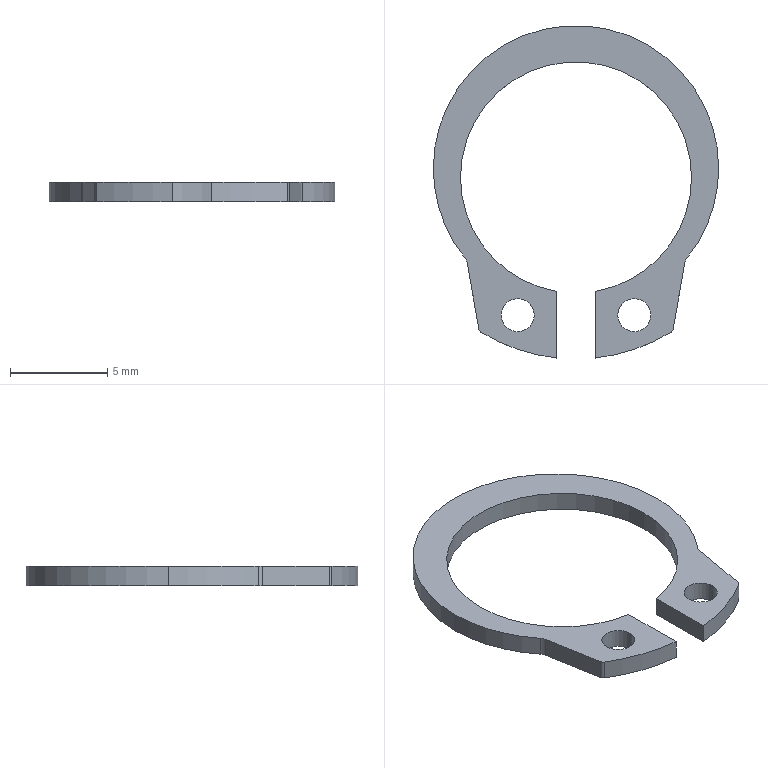Part | SolidWorks | features Extrusion 1 | 1 solid | 22 faces | box 14.7 x 17.116 x 1 mm | volume 75.123 mm3 | cylinder 16 | plane 6 | commonest cylinder face diameters 1.7 x4 11.9 x3 14.7 x3 0.4 x2 1 x2 18.7 x2
STEP:
#1=CARTESIAN_POINT('',(2.15,-7.562,0.5));
#2=VERTEX_POINT('',#1);
#3=CARTESIAN_POINT('',(3.85,-7.562,0.5));
#4=VERTEX_POINT('',#3);
#5=CARTESIAN_POINT('',(3.,-7.562,0.5));
#6=DIRECTION('',(0.,0.,1.));
#7=DIRECTION('',(-1.,0.,0.));
#8=AXIS2_PLACEMENT_3D('',#5,#6,#7);
#9=CIRCLE('',#8,0.85);
#10=EDGE_CURVE('',#2,#4,#9,.T.);
#11=ORIENTED_EDGE('',*,*,#10,.T.);
#12=CARTESIAN_POINT('',(3.85,-7.562,-0.5));
#13=VERTEX_POINT('',#12);
#14=CARTESIAN_POINT('',(3.85,-7.562,0.5));
#15=DIRECTION('',(0.,0.,-1.));
#16=VECTOR('',#15,1000.);
#17=LINE('',#14,#16);
#18=EDGE_CURVE('',#4,#13,#17,.T.);
#19=ORIENTED_EDGE('',*,*,#18,.T.);
#20=CARTESIAN_POINT('',(2.15,-7.562,-0.5));
#21=VERTEX_POINT('',#20);
#22=CARTESIAN_POINT('',(3.,-7.562,-0.5));
#23=DIRECTION('',(0.,0.,1.));
#24=DIRECTION('',(-1.,0.,0.));
#25=AXIS2_PLACEMENT_3D('',#22,#23,#24);
#26=CIRCLE('',#25,0.85);
#27=EDGE_CURVE('',#21,#13,#26,.T.);
#28=ORIENTED_EDGE('',*,*,#27,.F.);
#29=CARTESIAN_POINT('',(2.15,-7.562,0.5));
#30=DIRECTION('',(0.,0.,-1.));
#31=VECTOR('',#30,1000.);
#32=LINE('',#29,#31);
#33=EDGE_CURVE('',#2,#21,#32,.T.);
#34=ORIENTED_EDGE('',*,*,#33,.F.);
#35=EDGE_LOOP('',(#11,#19,#28,#34));
#36=FACE_OUTER_BOUND('',#35,.T.);
#37=CARTESIAN_POINT('',(3.,-7.562,0.5));
#38=DIRECTION('',(0.,0.,-1.));
#39=DIRECTION('',(-1.,0.,0.));
#40=AXIS2_PLACEMENT_3D('',#37,#38,#39);
#41=CYLINDRICAL_SURFACE('',#40,0.85);
#42=ADVANCED_FACE('',(#36),#41,.F.);
#43=CARTESIAN_POINT('',(-3.85,-7.562,0.5));
#44=VERTEX_POINT('',#43);
#45=CARTESIAN_POINT('',(-2.15,-7.562,0.5));
#46=VERTEX_POINT('',#45);
#47=CARTESIAN_POINT('',(-3.,-7.562,0.5));
#48=DIRECTION('',(0.,0.,1.));
#49=DIRECTION('',(1.,0.,0.));
#50=AXIS2_PLACEMENT_3D('',#47,#48,#49);
#51=CIRCLE('',#50,0.85);
#52=EDGE_CURVE('',#44,#46,#51,.T.);
#53=ORIENTED_EDGE('',*,*,#52,.T.);
#54=CARTESIAN_POINT('',(-2.15,-7.562,-0.5));
#55=VERTEX_POINT('',#54);
#56=CARTESIAN_POINT('',(-2.15,-7.562,0.5));
#57=DIRECTION('',(0.,0.,-1.));
#58=VECTOR('',#57,1000.);
#59=LINE('',#56,#58);
#60=EDGE_CURVE('',#46,#55,#59,.T.);
#61=ORIENTED_EDGE('',*,*,#60,.T.);
#62=CARTESIAN_POINT('',(-3.85,-7.562,-0.5));
#63=VERTEX_POINT('',#62);
#64=CARTESIAN_POINT('',(-3.,-7.562,-0.5));
#65=DIRECTION('',(0.,0.,1.));
#66=DIRECTION('',(1.,0.,0.));
#67=AXIS2_PLACEMENT_3D('',#64,#65,#66);
#68=CIRCLE('',#67,0.85);
#69=EDGE_CURVE('',#63,#55,#68,.T.);
#70=ORIENTED_EDGE('',*,*,#69,.F.);
#71=CARTESIAN_POINT('',(-3.85,-7.562,0.5));
#72=DIRECTION('',(0.,0.,-1.));
#73=VECTOR('',#72,1000.);
#74=LINE('',#71,#73);
#75=EDGE_CURVE('',#44,#63,#74,.T.);
#76=ORIENTED_EDGE('',*,*,#75,.F.);
#77=EDGE_LOOP('',(#53,#61,#70,#76));
#78=FACE_OUTER_BOUND('',#77,.T.);
#79=CARTESIAN_POINT('',(-3.,-7.562,0.5));
#80=DIRECTION('',(0.,0.,-1.));
#81=DIRECTION('',(-1.,0.,0.));
#82=AXIS2_PLACEMENT_3D('',#79,#80,#81);
#83=CYLINDRICAL_SURFACE('',#82,0.85);
#84=ADVANCED_FACE('',(#78),#83,.F.);
#85=CARTESIAN_POINT('',(7.35,0.,0.5));
#86=VERTEX_POINT('',#85);
#87=CARTESIAN_POINT('',(-7.35,0.,0.5));
#88=VERTEX_POINT('',#87);
#89=CARTESIAN_POINT('',(0.,0.,0.5));
#90=DIRECTION('',(0.,0.,1.));
#91=DIRECTION('',(1.,0.,0.));
#92=AXIS2_PLACEMENT_3D('',#89,#90,#91);
#93=CIRCLE('',#92,7.35);
#94=EDGE_CURVE('',#86,#88,#93,.T.);
#95=ORIENTED_EDGE('',*,*,#94,.F.);
#96=CARTESIAN_POINT('',(7.35,0.,-0.5));
#97=VERTEX_POINT('',#96);
#98=CARTESIAN_POINT('',(7.35,0.,0.5));
#99=DIRECTION('',(0.,0.,-1.));
#100=VECTOR('',#99,1000.);
#101=LINE('',#98,#100);
#102=EDGE_CURVE('',#86,#97,#101,.T.);
#103=ORIENTED_EDGE('',*,*,#102,.T.);
#104=CARTESIAN_POINT('',(-7.35,0.,-0.5));
#105=VERTEX_POINT('',#104);
#106=CARTESIAN_POINT('',(0.,0.,-0.5));
#107=DIRECTION('',(0.,0.,1.));
#108=DIRECTION('',(1.,0.,0.));
#109=AXIS2_PLACEMENT_3D('',#106,#107,#108);
#110=CIRCLE('',#109,7.35);
#111=EDGE_CURVE('',#97,#105,#110,.T.);
#112=ORIENTED_EDGE('',*,*,#111,.T.);
#113=CARTESIAN_POINT('',(-7.35,0.,0.5));
#114=DIRECTION('',(0.,0.,-1.));
#115=VECTOR('',#114,1000.);
#116=LINE('',#113,#115);
#117=EDGE_CURVE('',#88,#105,#116,.T.);
#118=ORIENTED_EDGE('',*,*,#117,.F.);
#119=EDGE_LOOP('',(#95,#103,#112,#118));
#120=FACE_OUTER_BOUND('',#119,.T.);
#121=CARTESIAN_POINT('',(0.,0.,0.5));
#122=DIRECTION('',(0.,0.,-1.));
#123=DIRECTION('',(-1.,0.,0.));
#124=AXIS2_PLACEMENT_3D('',#121,#122,#123);
#125=CYLINDRICAL_SURFACE('',#124,7.35);
#126=ADVANCED_FACE('',(#120),#125,.T.);
#127=CARTESIAN_POINT('',(-5.71,-4.628,0.5));
#128=VERTEX_POINT('',#127);
#129=CARTESIAN_POINT('',(0.,0.,0.5));
#130=DIRECTION('',(0.,0.,1.));
#131=DIRECTION('',(1.,0.,0.));
#132=AXIS2_PLACEMENT_3D('',#129,#130,#131);
#133=CIRCLE('',#132,7.35);
#134=EDGE_CURVE('',#88,#128,#133,.T.);
#135=ORIENTED_EDGE('',*,*,#134,.F.);
#136=ORIENTED_EDGE('',*,*,#117,.T.);
#137=CARTESIAN_POINT('',(-5.71,-4.628,-0.5));
#138=VERTEX_POINT('',#137);
#139=CARTESIAN_POINT('',(0.,0.,-0.5));
#140=DIRECTION('',(0.,0.,1.));
#141=DIRECTION('',(1.,0.,0.));
#142=AXIS2_PLACEMENT_3D('',#139,#140,#141);
#143=CIRCLE('',#142,7.35);
#144=EDGE_CURVE('',#105,#138,#143,.T.);
#145=ORIENTED_EDGE('',*,*,#144,.T.);
#146=CARTESIAN_POINT('',(-5.71,-4.628,0.5));
#147=DIRECTION('',(0.,0.,-1.));
#148=VECTOR('',#147,1000.);
#149=LINE('',#146,#148);
#150=EDGE_CURVE('',#128,#138,#149,.T.);
#151=ORIENTED_EDGE('',*,*,#150,.F.);
#152=EDGE_LOOP('',(#135,#136,#145,#151));
#153=FACE_OUTER_BOUND('',#152,.T.);
#154=CARTESIAN_POINT('',(0.,0.,0.5));
#155=DIRECTION('',(0.,0.,-1.));
#156=DIRECTION('',(-1.,0.,0.));
#157=AXIS2_PLACEMENT_3D('',#154,#155,#156);
#158=CYLINDRICAL_SURFACE('',#157,7.35);
#159=ADVANCED_FACE('',(#153),#158,.T.);
#160=CARTESIAN_POINT('',(5.95,-0.47,0.5));
#161=VERTEX_POINT('',#160);
#162=CARTESIAN_POINT('',(1.,-6.335,0.5));
#163=VERTEX_POINT('',#162);
#164=CARTESIAN_POINT('',(0.,-0.47,0.5));
#165=DIRECTION('',(0.,0.,-1.));
#166=DIRECTION('',(1.,0.,0.));
#167=AXIS2_PLACEMENT_3D('',#164,#165,#166);
#168=CIRCLE('',#167,5.95);
#169=EDGE_CURVE('',#161,#163,#168,.T.);
#170=ORIENTED_EDGE('',*,*,#169,.F.);
#171=CARTESIAN_POINT('',(5.95,-0.47,-0.5));
#172=VERTEX_POINT('',#171);
#173=CARTESIAN_POINT('',(5.95,-0.47,0.5));
#174=DIRECTION('',(0.,0.,-1.));
#175=VECTOR('',#174,1000.);
#176=LINE('',#173,#175);
#177=EDGE_CURVE('',#161,#172,#176,.T.);
#178=ORIENTED_EDGE('',*,*,#177,.T.);
#179=CARTESIAN_POINT('',(1.,-6.335,-0.5));
#180=VERTEX_POINT('',#179);
#181=CARTESIAN_POINT('',(0.,-0.47,-0.5));
#182=DIRECTION('',(0.,0.,-1.));
#183=DIRECTION('',(1.,0.,0.));
#184=AXIS2_PLACEMENT_3D('',#181,#182,#183);
#185=CIRCLE('',#184,5.95);
#186=EDGE_CURVE('',#172,#180,#185,.T.);
#187=ORIENTED_EDGE('',*,*,#186,.T.);
#188=CARTESIAN_POINT('',(1.,-6.335,0.5));
#189=DIRECTION('',(0.,0.,-1.));
#190=VECTOR('',#189,1000.);
#191=LINE('',#188,#190);
#192=EDGE_CURVE('',#163,#180,#191,.T.);
#193=ORIENTED_EDGE('',*,*,#192,.F.);
#194=EDGE_LOOP('',(#170,#178,#187,#193));
#195=FACE_OUTER_BOUND('',#194,.T.);
#196=CARTESIAN_POINT('',(0.,-0.47,0.5));
#197=DIRECTION('',(0.,0.,-1.));
#198=DIRECTION('',(-1.,0.,0.));
#199=AXIS2_PLACEMENT_3D('',#196,#197,#198);
#200=CYLINDRICAL_SURFACE('',#199,5.95);
#201=ADVANCED_FACE('',(#195),#200,.F.);
#202=ORIENTED_EDGE('',*,*,#177,.F.);
#203=CARTESIAN_POINT('',(-5.95,-0.47,0.5));
#204=VERTEX_POINT('',#203);
#205=CARTESIAN_POINT('',(0.,-0.47,0.5));
#206=DIRECTION('',(0.,0.,-1.));
#207=DIRECTION('',(1.,0.,0.));
#208=AXIS2_PLACEMENT_3D('',#205,#206,#207);
#209=CIRCLE('',#208,5.95);
#210=EDGE_CURVE('',#204,#161,#209,.T.);
#211=ORIENTED_EDGE('',*,*,#210,.F.);
#212=CARTESIAN_POINT('',(-5.95,-0.47,-0.5));
#213=VERTEX_POINT('',#212);
#214=CARTESIAN_POINT('',(-5.95,-0.47,0.5));
#215=DIRECTION('',(0.,0.,-1.));
#216=VECTOR('',#215,1000.);
#217=LINE('',#214,#216);
#218=EDGE_CURVE('',#204,#213,#217,.T.);
#219=ORIENTED_EDGE('',*,*,#218,.T.);
#220=CARTESIAN_POINT('',(0.,-0.47,-0.5));
#221=DIRECTION('',(0.,0.,-1.));
#222=DIRECTION('',(1.,0.,0.));
#223=AXIS2_PLACEMENT_3D('',#220,#221,#222);
#224=CIRCLE('',#223,5.95);
#225=EDGE_CURVE('',#213,#172,#224,.T.);
#226=ORIENTED_EDGE('',*,*,#225,.T.);
#227=EDGE_LOOP('',(#202,#211,#219,#226));
#228=FACE_OUTER_BOUND('',#227,.T.);
#229=CARTESIAN_POINT('',(0.,-0.47,0.5));
#230=DIRECTION('',(0.,0.,-1.));
#231=DIRECTION('',(-1.,0.,0.));
#232=AXIS2_PLACEMENT_3D('',#229,#230,#231);
#233=CYLINDRICAL_SURFACE('',#232,5.95);
#234=ADVANCED_FACE('',(#228),#233,.F.);
#235=ORIENTED_EDGE('',*,*,#52,.F.);
#236=CARTESIAN_POINT('',(-3.,-7.562,0.5));
#237=DIRECTION('',(0.,0.,1.));
#238=DIRECTION('',(1.,0.,0.));
#239=AXIS2_PLACEMENT_3D('',#236,#237,#238);
#240=CIRCLE('',#239,0.85);
#241=EDGE_CURVE('',#46,#44,#240,.T.);
#242=ORIENTED_EDGE('',*,*,#241,.F.);
#243=EDGE_LOOP('',(#235,#242));
#244=FACE_BOUND('',#243,.T.);
#245=CARTESIAN_POINT('',(-5.606,-4.856,0.5));
#246=VERTEX_POINT('',#245);
#247=CARTESIAN_POINT('',(-6.098,-4.943,0.5));
#248=DIRECTION('',(0.,0.,-1.));
#249=DIRECTION('',(1.,0.,0.));
#250=AXIS2_PLACEMENT_3D('',#247,#248,#249);
#251=CIRCLE('',#250,0.5);
#252=EDGE_CURVE('',#128,#246,#251,.T.);
#253=ORIENTED_EDGE('',*,*,#252,.T.);
#254=CARTESIAN_POINT('',(-5.,-8.293,0.5));
#255=VERTEX_POINT('',#254);
#256=CARTESIAN_POINT('',(-5.606,-4.856,0.5));
#257=DIRECTION('',(0.1736,-0.9848,0.));
#258=VECTOR('',#257,1000.);
#259=LINE('',#256,#258);
#260=EDGE_CURVE('',#246,#255,#259,.T.);
#261=ORIENTED_EDGE('',*,*,#260,.T.);
#262=CARTESIAN_POINT('',(-4.908,-8.428,0.5));
#263=VERTEX_POINT('',#262);
#264=CARTESIAN_POINT('',(-4.803,-8.258,0.5));
#265=DIRECTION('',(0.,0.,1.));
#266=DIRECTION('',(-1.,0.,0.));
#267=AXIS2_PLACEMENT_3D('',#264,#265,#266);
#268=CIRCLE('',#267,0.2);
#269=EDGE_CURVE('',#255,#263,#268,.T.);
#270=ORIENTED_EDGE('',*,*,#269,.T.);
#271=CARTESIAN_POINT('',(-1.,-9.766,0.5));
#272=VERTEX_POINT('',#271);
#273=CARTESIAN_POINT('',(0.,-0.47,0.5));
#274=DIRECTION('',(0.,0.,1.));
#275=DIRECTION('',(-1.,0.,0.));
#276=AXIS2_PLACEMENT_3D('',#273,#274,#275);
#277=CIRCLE('',#276,9.35);
#278=EDGE_CURVE('',#263,#272,#277,.T.);
#279=ORIENTED_EDGE('',*,*,#278,.T.);
#280=CARTESIAN_POINT('',(-1.,-6.335,0.5));
#281=VERTEX_POINT('',#280);
#282=CARTESIAN_POINT('',(-1.,-6.335,0.5));
#283=DIRECTION('',(0.,1.,0.));
#284=VECTOR('',#283,1000.);
#285=LINE('',#282,#284);
#286=EDGE_CURVE('',#272,#281,#285,.T.);
#287=ORIENTED_EDGE('',*,*,#286,.T.);
#288=CARTESIAN_POINT('',(0.,-0.47,0.5));
#289=DIRECTION('',(0.,0.,-1.));
#290=DIRECTION('',(1.,0.,0.));
#291=AXIS2_PLACEMENT_3D('',#288,#289,#290);
#292=CIRCLE('',#291,5.95);
#293=EDGE_CURVE('',#281,#204,#292,.T.);
#294=ORIENTED_EDGE('',*,*,#293,.T.);
#295=ORIENTED_EDGE('',*,*,#210,.T.);
#296=ORIENTED_EDGE('',*,*,#169,.T.);
#297=CARTESIAN_POINT('',(1.,-9.766,0.5));
#298=VERTEX_POINT('',#297);
#299=CARTESIAN_POINT('',(1.,-6.335,0.5));
#300=DIRECTION('',(0.,-1.,0.));
#301=VECTOR('',#300,1000.);
#302=LINE('',#299,#301);
#303=EDGE_CURVE('',#163,#298,#302,.T.);
#304=ORIENTED_EDGE('',*,*,#303,.T.);
#305=CARTESIAN_POINT('',(4.908,-8.428,0.5));
#306=VERTEX_POINT('',#305);
#307=CARTESIAN_POINT('',(0.,-0.47,0.5));
#308=DIRECTION('',(0.,0.,1.));
#309=DIRECTION('',(1.,0.,0.));
#310=AXIS2_PLACEMENT_3D('',#307,#308,#309);
#311=CIRCLE('',#310,9.35);
#312=EDGE_CURVE('',#298,#306,#311,.T.);
#313=ORIENTED_EDGE('',*,*,#312,.T.);
#314=CARTESIAN_POINT('',(5.,-8.293,0.5));
#315=VERTEX_POINT('',#314);
#316=CARTESIAN_POINT('',(4.803,-8.258,0.5));
#317=DIRECTION('',(0.,0.,1.));
#318=DIRECTION('',(1.,0.,0.));
#319=AXIS2_PLACEMENT_3D('',#316,#317,#318);
#320=CIRCLE('',#319,0.2);
#321=EDGE_CURVE('',#306,#315,#320,.T.);
#322=ORIENTED_EDGE('',*,*,#321,.T.);
#323=CARTESIAN_POINT('',(5.606,-4.856,0.5));
#324=VERTEX_POINT('',#323);
#325=CARTESIAN_POINT('',(5.606,-4.856,0.5));
#326=DIRECTION('',(0.1736,0.9848,0.));
#327=VECTOR('',#326,1000.);
#328=LINE('',#325,#327);
#329=EDGE_CURVE('',#315,#324,#328,.T.);
#330=ORIENTED_EDGE('',*,*,#329,.T.);
#331=CARTESIAN_POINT('',(5.71,-4.628,0.5));
#332=VERTEX_POINT('',#331);
#333=CARTESIAN_POINT('',(6.098,-4.943,0.5));
#334=DIRECTION('',(0.,0.,-1.));
#335=DIRECTION('',(-1.,0.,0.));
#336=AXIS2_PLACEMENT_3D('',#333,#334,#335);
#337=CIRCLE('',#336,0.5);
#338=EDGE_CURVE('',#324,#332,#337,.T.);
#339=ORIENTED_EDGE('',*,*,#338,.T.);
#340=CARTESIAN_POINT('',(0.,0.,0.5));
#341=DIRECTION('',(0.,0.,1.));
#342=DIRECTION('',(1.,0.,0.));
#343=AXIS2_PLACEMENT_3D('',#340,#341,#342);
#344=CIRCLE('',#343,7.35);
#345=EDGE_CURVE('',#332,#86,#344,.T.);
#346=ORIENTED_EDGE('',*,*,#345,.T.);
#347=ORIENTED_EDGE('',*,*,#94,.T.);
#348=ORIENTED_EDGE('',*,*,#134,.T.);
#349=EDGE_LOOP('',(#253,#261,#270,#279,#287,#294,#295,#296,#304,#313,#322,#330,#339,#346,#347,#348));
#350=FACE_OUTER_BOUND('',#349,.T.);
#351=ORIENTED_EDGE('',*,*,#10,.F.);
#352=CARTESIAN_POINT('',(3.,-7.562,0.5));
#353=DIRECTION('',(0.,0.,1.));
#354=DIRECTION('',(-1.,0.,0.));
#355=AXIS2_PLACEMENT_3D('',#352,#353,#354);
#356=CIRCLE('',#355,0.85);
#357=EDGE_CURVE('',#4,#2,#356,.T.);
#358=ORIENTED_EDGE('',*,*,#357,.F.);
#359=EDGE_LOOP('',(#351,#358));
#360=FACE_BOUND('',#359,.T.);
#361=CARTESIAN_POINT('',(-6.098,-4.943,0.5));
#362=DIRECTION('',(0.,0.,1.));
#363=DIRECTION('',(1.,0.,0.));
#364=AXIS2_PLACEMENT_3D('',#361,#362,#363);
#365=PLANE('',#364);
#366=ADVANCED_FACE('',(#244,#350,#360),#365,.T.);
#367=ORIENTED_EDGE('',*,*,#150,.T.);
#368=CARTESIAN_POINT('',(-5.606,-4.856,-0.5));
#369=VERTEX_POINT('',#368);
#370=CARTESIAN_POINT('',(-6.098,-4.943,-0.5));
#371=DIRECTION('',(0.,0.,-1.));
#372=DIRECTION('',(1.,0.,0.));
#373=AXIS2_PLACEMENT_3D('',#370,#371,#372);
#374=CIRCLE('',#373,0.5);
#375=EDGE_CURVE('',#138,#369,#374,.T.);
#376=ORIENTED_EDGE('',*,*,#375,.T.);
#377=CARTESIAN_POINT('',(-5.606,-4.856,0.5));
#378=DIRECTION('',(0.,0.,-1.));
#379=VECTOR('',#378,1000.);
#380=LINE('',#377,#379);
#381=EDGE_CURVE('',#246,#369,#380,.T.);
#382=ORIENTED_EDGE('',*,*,#381,.F.);
#383=ORIENTED_EDGE('',*,*,#252,.F.);
#384=EDGE_LOOP('',(#367,#376,#382,#383));
#385=FACE_OUTER_BOUND('',#384,.T.);
#386=CARTESIAN_POINT('',(-6.098,-4.943,0.5));
#387=DIRECTION('',(0.,0.,-1.));
#388=DIRECTION('',(-1.,0.,0.));
#389=AXIS2_PLACEMENT_3D('',#386,#387,#388);
#390=CYLINDRICAL_SURFACE('',#389,0.5);
#391=ADVANCED_FACE('',(#385),#390,.F.);
#392=ORIENTED_EDGE('',*,*,#381,.T.);
#393=CARTESIAN_POINT('',(-5.,-8.293,-0.5));
#394=VERTEX_POINT('',#393);
#395=CARTESIAN_POINT('',(-5.606,-4.856,-0.5));
#396=DIRECTION('',(0.1736,-0.9848,0.));
#397=VECTOR('',#396,1000.);
#398=LINE('',#395,#397);
#399=EDGE_CURVE('',#369,#394,#398,.T.);
#400=ORIENTED_EDGE('',*,*,#399,.T.);
#401=CARTESIAN_POINT('',(-5.,-8.293,0.5));
#402=DIRECTION('',(0.,0.,-1.));
#403=VECTOR('',#402,1000.);
#404=LINE('',#401,#403);
#405=EDGE_CURVE('',#255,#394,#404,.T.);
#406=ORIENTED_EDGE('',*,*,#405,.F.);
#407=ORIENTED_EDGE('',*,*,#260,.F.);
#408=EDGE_LOOP('',(#392,#400,#406,#407));
#409=FACE_OUTER_BOUND('',#408,.T.);
#410=CARTESIAN_POINT('',(-5.606,-4.856,0.5));
#411=DIRECTION('',(0.9848,0.1736,0.));
#412=DIRECTION('',(-0.1736,0.9848,0.));
#413=AXIS2_PLACEMENT_3D('',#410,#411,#412);
#414=PLANE('',#413);
#415=ADVANCED_FACE('',(#409),#414,.F.);
#416=ORIENTED_EDGE('',*,*,#405,.T.);
#417=CARTESIAN_POINT('',(-4.908,-8.428,-0.5));
#418=VERTEX_POINT('',#417);
#419=CARTESIAN_POINT('',(-4.803,-8.258,-0.5));
#420=DIRECTION('',(0.,0.,1.));
#421=DIRECTION('',(-1.,0.,0.));
#422=AXIS2_PLACEMENT_3D('',#419,#420,#421);
#423=CIRCLE('',#422,0.2);
#424=EDGE_CURVE('',#394,#418,#423,.T.);
#425=ORIENTED_EDGE('',*,*,#424,.T.);
#426=CARTESIAN_POINT('',(-4.908,-8.428,0.5));
#427=DIRECTION('',(0.,0.,-1.));
#428=VECTOR('',#427,1000.);
#429=LINE('',#426,#428);
#430=EDGE_CURVE('',#263,#418,#429,.T.);
#431=ORIENTED_EDGE('',*,*,#430,.F.);
#432=ORIENTED_EDGE('',*,*,#269,.F.);
#433=EDGE_LOOP('',(#416,#425,#431,#432));
#434=FACE_OUTER_BOUND('',#433,.T.);
#435=CARTESIAN_POINT('',(-4.803,-8.258,0.5));
#436=DIRECTION('',(0.,0.,-1.));
#437=DIRECTION('',(-1.,0.,0.));
#438=AXIS2_PLACEMENT_3D('',#435,#436,#437);
#439=CYLINDRICAL_SURFACE('',#438,0.2);
#440=ADVANCED_FACE('',(#434),#439,.T.);
#441=ORIENTED_EDGE('',*,*,#430,.T.);
#442=CARTESIAN_POINT('',(-1.,-9.766,-0.5));
#443=VERTEX_POINT('',#442);
#444=CARTESIAN_POINT('',(0.,-0.47,-0.5));
#445=DIRECTION('',(0.,0.,1.));
#446=DIRECTION('',(-1.,0.,0.));
#447=AXIS2_PLACEMENT_3D('',#444,#445,#446);
#448=CIRCLE('',#447,9.35);
#449=EDGE_CURVE('',#418,#443,#448,.T.);
#450=ORIENTED_EDGE('',*,*,#449,.T.);
#451=CARTESIAN_POINT('',(-1.,-9.766,0.5));
#452=DIRECTION('',(0.,0.,-1.));
#453=VECTOR('',#452,1000.);
#454=LINE('',#451,#453);
#455=EDGE_CURVE('',#272,#443,#454,.T.);
#456=ORIENTED_EDGE('',*,*,#455,.F.);
#457=ORIENTED_EDGE('',*,*,#278,.F.);
#458=EDGE_LOOP('',(#441,#450,#456,#457));
#459=FACE_OUTER_BOUND('',#458,.T.);
#460=CARTESIAN_POINT('',(0.,-0.47,0.5));
#461=DIRECTION('',(0.,0.,-1.));
#462=DIRECTION('',(-1.,0.,0.));
#463=AXIS2_PLACEMENT_3D('',#460,#461,#462);
#464=CYLINDRICAL_SURFACE('',#463,9.35);
#465=ADVANCED_FACE('',(#459),#464,.T.);
#466=ORIENTED_EDGE('',*,*,#455,.T.);
#467=CARTESIAN_POINT('',(-1.,-6.335,-0.5));
#468=VERTEX_POINT('',#467);
#469=CARTESIAN_POINT('',(-1.,-6.335,-0.5));
#470=DIRECTION('',(0.,1.,0.));
#471=VECTOR('',#470,1000.);
#472=LINE('',#469,#471);
#473=EDGE_CURVE('',#443,#468,#472,.T.);
#474=ORIENTED_EDGE('',*,*,#473,.T.);
#475=CARTESIAN_POINT('',(-1.,-6.335,0.5));
#476=DIRECTION('',(0.,0.,-1.));
#477=VECTOR('',#476,1000.);
#478=LINE('',#475,#477);
#479=EDGE_CURVE('',#281,#468,#478,.T.);
#480=ORIENTED_EDGE('',*,*,#479,.F.);
#481=ORIENTED_EDGE('',*,*,#286,.F.);
#482=EDGE_LOOP('',(#466,#474,#480,#481));
#483=FACE_OUTER_BOUND('',#482,.T.);
#484=CARTESIAN_POINT('',(-1.,-6.335,0.5));
#485=DIRECTION('',(-1.,0.,0.));
#486=DIRECTION('',(0.,-1.,0.));
#487=AXIS2_PLACEMENT_3D('',#484,#485,#486);
#488=PLANE('',#487);
#489=ADVANCED_FACE('',(#483),#488,.F.);
#490=ORIENTED_EDGE('',*,*,#218,.F.);
#491=ORIENTED_EDGE('',*,*,#293,.F.);
#492=ORIENTED_EDGE('',*,*,#479,.T.);
#493=CARTESIAN_POINT('',(0.,-0.47,-0.5));
#494=DIRECTION('',(0.,0.,-1.));
#495=DIRECTION('',(1.,0.,0.));
#496=AXIS2_PLACEMENT_3D('',#493,#494,#495);
#497=CIRCLE('',#496,5.95);
#498=EDGE_CURVE('',#468,#213,#497,.T.);
#499=ORIENTED_EDGE('',*,*,#498,.T.);
#500=EDGE_LOOP('',(#490,#491,#492,#499));
#501=FACE_OUTER_BOUND('',#500,.T.);
#502=CARTESIAN_POINT('',(0.,-0.47,0.5));
#503=DIRECTION('',(0.,0.,-1.));
#504=DIRECTION('',(-1.,0.,0.));
#505=AXIS2_PLACEMENT_3D('',#502,#503,#504);
#506=CYLINDRICAL_SURFACE('',#505,5.95);
#507=ADVANCED_FACE('',(#501),#506,.F.);
#508=ORIENTED_EDGE('',*,*,#192,.T.);
#509=CARTESIAN_POINT('',(1.,-9.766,-0.5));
#510=VERTEX_POINT('',#509);
#511=CARTESIAN_POINT('',(1.,-6.335,-0.5));
#512=DIRECTION('',(0.,-1.,0.));
#513=VECTOR('',#512,1000.);
#514=LINE('',#511,#513);
#515=EDGE_CURVE('',#180,#510,#514,.T.);
#516=ORIENTED_EDGE('',*,*,#515,.T.);
#517=CARTESIAN_POINT('',(1.,-9.766,0.5));
#518=DIRECTION('',(0.,0.,-1.));
#519=VECTOR('',#518,1000.);
#520=LINE('',#517,#519);
#521=EDGE_CURVE('',#298,#510,#520,.T.);
#522=ORIENTED_EDGE('',*,*,#521,.F.);
#523=ORIENTED_EDGE('',*,*,#303,.F.);
#524=EDGE_LOOP('',(#508,#516,#522,#523));
#525=FACE_OUTER_BOUND('',#524,.T.);
#526=CARTESIAN_POINT('',(1.,-6.335,0.5));
#527=DIRECTION('',(1.,0.,0.));
#528=DIRECTION('',(0.,1.,0.));
#529=AXIS2_PLACEMENT_3D('',#526,#527,#528);
#530=PLANE('',#529);
#531=ADVANCED_FACE('',(#525),#530,.F.);
#532=ORIENTED_EDGE('',*,*,#521,.T.);
#533=CARTESIAN_POINT('',(4.908,-8.428,-0.5));
#534=VERTEX_POINT('',#533);
#535=CARTESIAN_POINT('',(0.,-0.47,-0.5));
#536=DIRECTION('',(0.,0.,1.));
#537=DIRECTION('',(1.,0.,0.));
#538=AXIS2_PLACEMENT_3D('',#535,#536,#537);
#539=CIRCLE('',#538,9.35);
#540=EDGE_CURVE('',#510,#534,#539,.T.);
#541=ORIENTED_EDGE('',*,*,#540,.T.);
#542=CARTESIAN_POINT('',(4.908,-8.428,0.5));
#543=DIRECTION('',(0.,0.,-1.));
#544=VECTOR('',#543,1000.);
#545=LINE('',#542,#544);
#546=EDGE_CURVE('',#306,#534,#545,.T.);
#547=ORIENTED_EDGE('',*,*,#546,.F.);
#548=ORIENTED_EDGE('',*,*,#312,.F.);
#549=EDGE_LOOP('',(#532,#541,#547,#548));
#550=FACE_OUTER_BOUND('',#549,.T.);
#551=CARTESIAN_POINT('',(0.,-0.47,0.5));
#552=DIRECTION('',(0.,0.,-1.));
#553=DIRECTION('',(-1.,0.,0.));
#554=AXIS2_PLACEMENT_3D('',#551,#552,#553);
#555=CYLINDRICAL_SURFACE('',#554,9.35);
#556=ADVANCED_FACE('',(#550),#555,.T.);
#557=ORIENTED_EDGE('',*,*,#546,.T.);
#558=CARTESIAN_POINT('',(5.,-8.293,-0.5));
#559=VERTEX_POINT('',#558);
#560=CARTESIAN_POINT('',(4.803,-8.258,-0.5));
#561=DIRECTION('',(0.,0.,1.));
#562=DIRECTION('',(1.,0.,0.));
#563=AXIS2_PLACEMENT_3D('',#560,#561,#562);
#564=CIRCLE('',#563,0.2);
#565=EDGE_CURVE('',#534,#559,#564,.T.);
#566=ORIENTED_EDGE('',*,*,#565,.T.);
#567=CARTESIAN_POINT('',(5.,-8.293,0.5));
#568=DIRECTION('',(0.,0.,-1.));
#569=VECTOR('',#568,1000.);
#570=LINE('',#567,#569);
#571=EDGE_CURVE('',#315,#559,#570,.T.);
#572=ORIENTED_EDGE('',*,*,#571,.F.);
#573=ORIENTED_EDGE('',*,*,#321,.F.);
#574=EDGE_LOOP('',(#557,#566,#572,#573));
#575=FACE_OUTER_BOUND('',#574,.T.);
#576=CARTESIAN_POINT('',(4.803,-8.258,0.5));
#577=DIRECTION('',(0.,0.,-1.));
#578=DIRECTION('',(-1.,0.,0.));
#579=AXIS2_PLACEMENT_3D('',#576,#577,#578);
#580=CYLINDRICAL_SURFACE('',#579,0.2);
#581=ADVANCED_FACE('',(#575),#580,.T.);
#582=ORIENTED_EDGE('',*,*,#571,.T.);
#583=CARTESIAN_POINT('',(5.606,-4.856,-0.5));
#584=VERTEX_POINT('',#583);
#585=CARTESIAN_POINT('',(5.606,-4.856,-0.5));
#586=DIRECTION('',(0.1736,0.9848,0.));
#587=VECTOR('',#586,1000.);
#588=LINE('',#585,#587);
#589=EDGE_CURVE('',#559,#584,#588,.T.);
#590=ORIENTED_EDGE('',*,*,#589,.T.);
#591=CARTESIAN_POINT('',(5.606,-4.856,0.5));
#592=DIRECTION('',(0.,0.,-1.));
#593=VECTOR('',#592,1000.);
#594=LINE('',#591,#593);
#595=EDGE_CURVE('',#324,#584,#594,.T.);
#596=ORIENTED_EDGE('',*,*,#595,.F.);
#597=ORIENTED_EDGE('',*,*,#329,.F.);
#598=EDGE_LOOP('',(#582,#590,#596,#597));
#599=FACE_OUTER_BOUND('',#598,.T.);
#600=CARTESIAN_POINT('',(5.606,-4.856,0.5));
#601=DIRECTION('',(-0.9848,0.1736,0.));
#602=DIRECTION('',(-0.1736,-0.9848,0.));
#603=AXIS2_PLACEMENT_3D('',#600,#601,#602);
#604=PLANE('',#603);
#605=ADVANCED_FACE('',(#599),#604,.F.);
#606=ORIENTED_EDGE('',*,*,#595,.T.);
#607=CARTESIAN_POINT('',(5.71,-4.628,-0.5));
#608=VERTEX_POINT('',#607);
#609=CARTESIAN_POINT('',(6.098,-4.943,-0.5));
#610=DIRECTION('',(0.,0.,-1.));
#611=DIRECTION('',(-1.,0.,0.));
#612=AXIS2_PLACEMENT_3D('',#609,#610,#611);
#613=CIRCLE('',#612,0.5);
#614=EDGE_CURVE('',#584,#608,#613,.T.);
#615=ORIENTED_EDGE('',*,*,#614,.T.);
#616=CARTESIAN_POINT('',(5.71,-4.628,0.5));
#617=DIRECTION('',(0.,0.,-1.));
#618=VECTOR('',#617,1000.);
#619=LINE('',#616,#618);
#620=EDGE_CURVE('',#332,#608,#619,.T.);
#621=ORIENTED_EDGE('',*,*,#620,.F.);
#622=ORIENTED_EDGE('',*,*,#338,.F.);
#623=EDGE_LOOP('',(#606,#615,#621,#622));
#624=FACE_OUTER_BOUND('',#623,.T.);
#625=CARTESIAN_POINT('',(6.098,-4.943,0.5));
#626=DIRECTION('',(0.,0.,-1.));
#627=DIRECTION('',(-1.,0.,0.));
#628=AXIS2_PLACEMENT_3D('',#625,#626,#627);
#629=CYLINDRICAL_SURFACE('',#628,0.5);
#630=ADVANCED_FACE('',(#624),#629,.F.);
#631=ORIENTED_EDGE('',*,*,#102,.F.);
#632=ORIENTED_EDGE('',*,*,#345,.F.);
#633=ORIENTED_EDGE('',*,*,#620,.T.);
#634=CARTESIAN_POINT('',(0.,0.,-0.5));
#635=DIRECTION('',(0.,0.,1.));
#636=DIRECTION('',(1.,0.,0.));
#637=AXIS2_PLACEMENT_3D('',#634,#635,#636);
#638=CIRCLE('',#637,7.35);
#639=EDGE_CURVE('',#608,#97,#638,.T.);
#640=ORIENTED_EDGE('',*,*,#639,.T.);
#641=EDGE_LOOP('',(#631,#632,#633,#640));
#642=FACE_OUTER_BOUND('',#641,.T.);
#643=CARTESIAN_POINT('',(0.,0.,0.5));
#644=DIRECTION('',(0.,0.,-1.));
#645=DIRECTION('',(-1.,0.,0.));
#646=AXIS2_PLACEMENT_3D('',#643,#644,#645);
#647=CYLINDRICAL_SURFACE('',#646,7.35);
#648=ADVANCED_FACE('',(#642),#647,.T.);
#649=ORIENTED_EDGE('',*,*,#60,.F.);
#650=ORIENTED_EDGE('',*,*,#241,.T.);
#651=ORIENTED_EDGE('',*,*,#75,.T.);
#652=CARTESIAN_POINT('',(-3.,-7.562,-0.5));
#653=DIRECTION('',(0.,0.,1.));
#654=DIRECTION('',(1.,0.,0.));
#655=AXIS2_PLACEMENT_3D('',#652,#653,#654);
#656=CIRCLE('',#655,0.85);
#657=EDGE_CURVE('',#55,#63,#656,.T.);
#658=ORIENTED_EDGE('',*,*,#657,.F.);
#659=EDGE_LOOP('',(#649,#650,#651,#658));
#660=FACE_OUTER_BOUND('',#659,.T.);
#661=CARTESIAN_POINT('',(-3.,-7.562,0.5));
#662=DIRECTION('',(0.,0.,-1.));
#663=DIRECTION('',(-1.,0.,0.));
#664=AXIS2_PLACEMENT_3D('',#661,#662,#663);
#665=CYLINDRICAL_SURFACE('',#664,0.85);
#666=ADVANCED_FACE('',(#660),#665,.F.);
#667=ORIENTED_EDGE('',*,*,#18,.F.);
#668=ORIENTED_EDGE('',*,*,#357,.T.);
#669=ORIENTED_EDGE('',*,*,#33,.T.);
#670=CARTESIAN_POINT('',(3.,-7.562,-0.5));
#671=DIRECTION('',(0.,0.,1.));
#672=DIRECTION('',(-1.,0.,0.));
#673=AXIS2_PLACEMENT_3D('',#670,#671,#672);
#674=CIRCLE('',#673,0.85);
#675=EDGE_CURVE('',#13,#21,#674,.T.);
#676=ORIENTED_EDGE('',*,*,#675,.F.);
#677=EDGE_LOOP('',(#667,#668,#669,#676));
#678=FACE_OUTER_BOUND('',#677,.T.);
#679=CARTESIAN_POINT('',(3.,-7.562,0.5));
#680=DIRECTION('',(0.,0.,-1.));
#681=DIRECTION('',(-1.,0.,0.));
#682=AXIS2_PLACEMENT_3D('',#679,#680,#681);
#683=CYLINDRICAL_SURFACE('',#682,0.85);
#684=ADVANCED_FACE('',(#678),#683,.F.);
#685=ORIENTED_EDGE('',*,*,#27,.T.);
#686=ORIENTED_EDGE('',*,*,#675,.T.);
#687=EDGE_LOOP('',(#685,#686));
#688=FACE_BOUND('',#687,.T.);
#689=ORIENTED_EDGE('',*,*,#69,.T.);
#690=ORIENTED_EDGE('',*,*,#657,.T.);
#691=EDGE_LOOP('',(#689,#690));
#692=FACE_BOUND('',#691,.T.);
#693=ORIENTED_EDGE('',*,*,#375,.F.);
#694=ORIENTED_EDGE('',*,*,#144,.F.);
#695=ORIENTED_EDGE('',*,*,#111,.F.);
#696=ORIENTED_EDGE('',*,*,#639,.F.);
#697=ORIENTED_EDGE('',*,*,#614,.F.);
#698=ORIENTED_EDGE('',*,*,#589,.F.);
#699=ORIENTED_EDGE('',*,*,#565,.F.);
#700=ORIENTED_EDGE('',*,*,#540,.F.);
#701=ORIENTED_EDGE('',*,*,#515,.F.);
#702=ORIENTED_EDGE('',*,*,#186,.F.);
#703=ORIENTED_EDGE('',*,*,#225,.F.);
#704=ORIENTED_EDGE('',*,*,#498,.F.);
#705=ORIENTED_EDGE('',*,*,#473,.F.);
#706=ORIENTED_EDGE('',*,*,#449,.F.);
#707=ORIENTED_EDGE('',*,*,#424,.F.);
#708=ORIENTED_EDGE('',*,*,#399,.F.);
#709=EDGE_LOOP('',(#693,#694,#695,#696,#697,#698,#699,#700,#701,#702,#703,#704,#705,#706,#707,#708));
#710=FACE_OUTER_BOUND('',#709,.T.);
#711=CARTESIAN_POINT('',(-6.098,-4.943,-0.5));
#712=DIRECTION('',(0.,0.,1.));
#713=DIRECTION('',(1.,0.,0.));
#714=AXIS2_PLACEMENT_3D('',#711,#712,#713);
#715=PLANE('',#714);
#716=ADVANCED_FACE('',(#688,#692,#710),#715,.F.);
#717=CLOSED_SHELL('',(#42,#84,#126,#159,#201,#234,#366,#391,#415,#440,#465,#489,#507,#531,#556,#581,#605,#630,#648,#666,#684,#716));
#718=MANIFOLD_SOLID_BREP('',#717);
#719=CARTESIAN_POINT('',(0.,0.,0.));
#720=DIRECTION('',(0.,0.,1.));
#721=DIRECTION('',(1.,0.,0.));
#722=AXIS2_PLACEMENT_3D('',#719,#720,#721);
#723=(LENGTH_UNIT()NAMED_UNIT(*)SI_UNIT(.MILLI.,.METRE.));
#724=UNCERTAINTY_MEASURE_WITH_UNIT(LENGTH_MEASURE(0.00001),#723,'','');
#725=(NAMED_UNIT(*)PLANE_ANGLE_UNIT()SI_UNIT($,.RADIAN.));
#726=(NAMED_UNIT(*)SI_UNIT($,.STERADIAN.)SOLID_ANGLE_UNIT());
#727=(GEOMETRIC_REPRESENTATION_CONTEXT(3)GLOBAL_UNCERTAINTY_ASSIGNED_CONTEXT((#724))GLOBAL_UNIT_ASSIGNED_CONTEXT((#723,#725,#726))REPRESENTATION_CONTEXT('',''));
#728=ADVANCED_BREP_SHAPE_REPRESENTATION('',(#718,#722),#727);